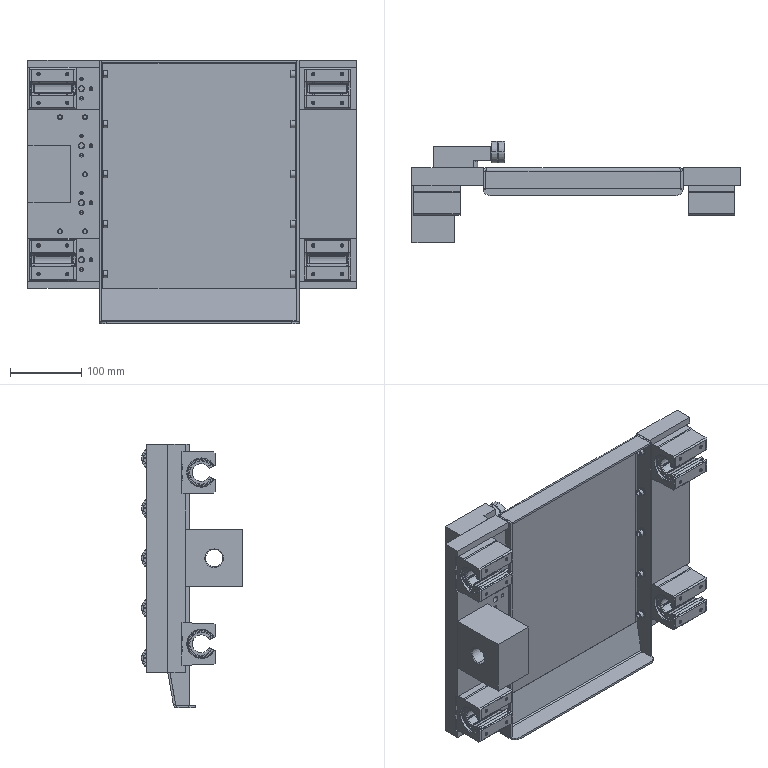Part | SolidWorks | 257 solids | 6436 faces | volume 3227627 mm3 | plane 2612 | cylinder 1540 | sphere 1528 | torus 580 | cone 172 | spline 4 | commonest cylinder face diameters 19 x190 21 x190 7 x112 10 x99 13 x76 21.25 x68